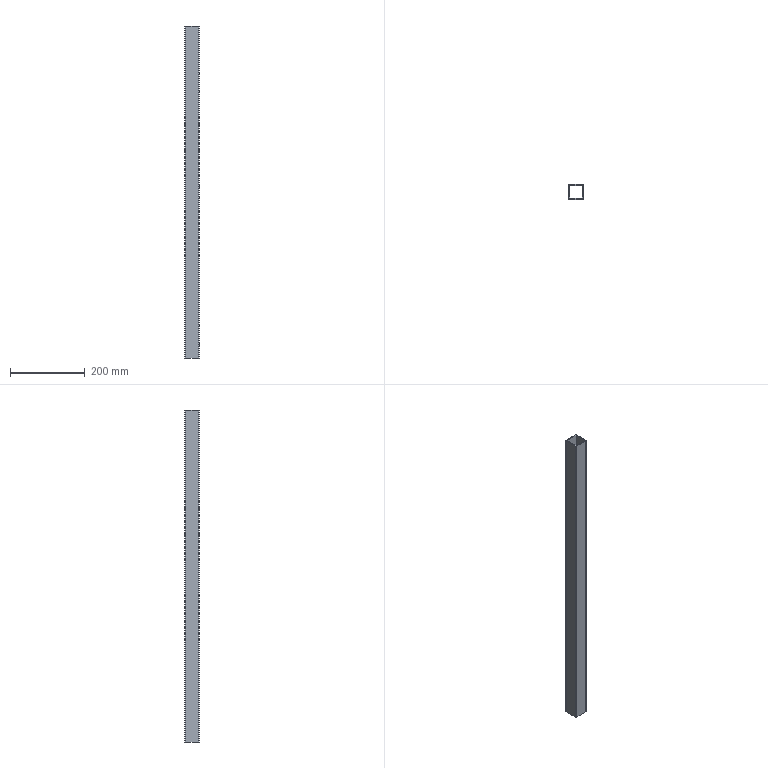Part | STEP file | X77-04201 | 1 solid | 26 faces | box 40 x 40 x 890 mm | volume 388035 mm3 | cylinder 16 | plane 10 | commonest cylinder face diameters 4.2 x12 6 x4
STEP:
#1=CARTESIAN_POINT('',(17.,12.,83.8));
#2=VERTEX_POINT('',#1);
#3=CARTESIAN_POINT('',(17.,12.,88.));
#4=VERTEX_POINT('',#3);
#5=CARTESIAN_POINT('',(17.,12.,85.9));
#6=DIRECTION('',(-1.,0.,0.));
#7=DIRECTION('',(0.,0.,1.));
#8=AXIS2_PLACEMENT_3D('',#5,#6,#7);
#9=CIRCLE('',#8,2.1);
#10=EDGE_CURVE('',#2,#4,#9,.T.);
#11=ORIENTED_EDGE('',*,*,#10,.T.);
#12=CARTESIAN_POINT('',(20.,12.,88.));
#13=VERTEX_POINT('',#12);
#14=CARTESIAN_POINT('',(20.,12.,88.));
#15=DIRECTION('',(1.,0.,0.));
#16=VECTOR('',#15,1000.);
#17=LINE('',#14,#16);
#18=EDGE_CURVE('',#4,#13,#17,.T.);
#19=ORIENTED_EDGE('',*,*,#18,.T.);
#20=CARTESIAN_POINT('',(20.,12.,83.8));
#21=VERTEX_POINT('',#20);
#22=CARTESIAN_POINT('',(20.,12.,85.9));
#23=DIRECTION('',(1.,0.,0.));
#24=DIRECTION('',(0.,0.,-1.));
#25=AXIS2_PLACEMENT_3D('',#22,#23,#24);
#26=CIRCLE('',#25,2.1);
#27=EDGE_CURVE('',#13,#21,#26,.T.);
#28=ORIENTED_EDGE('',*,*,#27,.T.);
#29=CARTESIAN_POINT('',(20.,12.,83.8));
#30=DIRECTION('',(1.,0.,0.));
#31=VECTOR('',#30,1000.);
#32=LINE('',#29,#31);
#33=EDGE_CURVE('',#2,#21,#32,.T.);
#34=ORIENTED_EDGE('',*,*,#33,.F.);
#35=EDGE_LOOP('',(#11,#19,#28,#34));
#36=FACE_OUTER_BOUND('',#35,.T.);
#37=CARTESIAN_POINT('',(20.,12.,85.9));
#38=DIRECTION('',(1.,0.,0.));
#39=DIRECTION('',(0.,0.,-1.));
#40=AXIS2_PLACEMENT_3D('',#37,#38,#39);
#41=CYLINDRICAL_SURFACE('',#40,2.1);
#42=ADVANCED_FACE('',(#36),#41,.F.);
#43=CARTESIAN_POINT('',(17.,-12.,33.8));
#44=VERTEX_POINT('',#43);
#45=CARTESIAN_POINT('',(17.,-12.,38.));
#46=VERTEX_POINT('',#45);
#47=CARTESIAN_POINT('',(17.,-12.,35.9));
#48=DIRECTION('',(-1.,0.,0.));
#49=DIRECTION('',(0.,0.,1.));
#50=AXIS2_PLACEMENT_3D('',#47,#48,#49);
#51=CIRCLE('',#50,2.1);
#52=EDGE_CURVE('',#44,#46,#51,.T.);
#53=ORIENTED_EDGE('',*,*,#52,.T.);
#54=CARTESIAN_POINT('',(20.,-12.,38.));
#55=VERTEX_POINT('',#54);
#56=CARTESIAN_POINT('',(20.,-12.,38.));
#57=DIRECTION('',(1.,0.,0.));
#58=VECTOR('',#57,1000.);
#59=LINE('',#56,#58);
#60=EDGE_CURVE('',#46,#55,#59,.T.);
#61=ORIENTED_EDGE('',*,*,#60,.T.);
#62=CARTESIAN_POINT('',(20.,-12.,33.8));
#63=VERTEX_POINT('',#62);
#64=CARTESIAN_POINT('',(20.,-12.,35.9));
#65=DIRECTION('',(1.,0.,0.));
#66=DIRECTION('',(0.,0.,-1.));
#67=AXIS2_PLACEMENT_3D('',#64,#65,#66);
#68=CIRCLE('',#67,2.1);
#69=EDGE_CURVE('',#55,#63,#68,.T.);
#70=ORIENTED_EDGE('',*,*,#69,.T.);
#71=CARTESIAN_POINT('',(20.,-12.,33.8));
#72=DIRECTION('',(1.,0.,0.));
#73=VECTOR('',#72,1000.);
#74=LINE('',#71,#73);
#75=EDGE_CURVE('',#44,#63,#74,.T.);
#76=ORIENTED_EDGE('',*,*,#75,.F.);
#77=EDGE_LOOP('',(#53,#61,#70,#76));
#78=FACE_OUTER_BOUND('',#77,.T.);
#79=CARTESIAN_POINT('',(20.,-12.,35.9));
#80=DIRECTION('',(1.,0.,0.));
#81=DIRECTION('',(0.,0.,-1.));
#82=AXIS2_PLACEMENT_3D('',#79,#80,#81);
#83=CYLINDRICAL_SURFACE('',#82,2.1);
#84=ADVANCED_FACE('',(#78),#83,.F.);
#85=CARTESIAN_POINT('',(17.,12.,762.));
#86=VERTEX_POINT('',#85);
#87=CARTESIAN_POINT('',(17.,12.,766.2));
#88=VERTEX_POINT('',#87);
#89=CARTESIAN_POINT('',(17.,12.,764.1));
#90=DIRECTION('',(-1.,0.,0.));
#91=DIRECTION('',(0.,0.,1.));
#92=AXIS2_PLACEMENT_3D('',#89,#90,#91);
#93=CIRCLE('',#92,2.1);
#94=EDGE_CURVE('',#86,#88,#93,.T.);
#95=ORIENTED_EDGE('',*,*,#94,.T.);
#96=CARTESIAN_POINT('',(20.,12.,766.2));
#97=VERTEX_POINT('',#96);
#98=CARTESIAN_POINT('',(20.,12.,766.2));
#99=DIRECTION('',(1.,0.,0.));
#100=VECTOR('',#99,1000.);
#101=LINE('',#98,#100);
#102=EDGE_CURVE('',#88,#97,#101,.T.);
#103=ORIENTED_EDGE('',*,*,#102,.T.);
#104=CARTESIAN_POINT('',(20.,12.,762.));
#105=VERTEX_POINT('',#104);
#106=CARTESIAN_POINT('',(20.,12.,764.1));
#107=DIRECTION('',(1.,0.,0.));
#108=DIRECTION('',(0.,0.,-1.));
#109=AXIS2_PLACEMENT_3D('',#106,#107,#108);
#110=CIRCLE('',#109,2.1);
#111=EDGE_CURVE('',#97,#105,#110,.T.);
#112=ORIENTED_EDGE('',*,*,#111,.T.);
#113=CARTESIAN_POINT('',(20.,12.,762.));
#114=DIRECTION('',(1.,0.,0.));
#115=VECTOR('',#114,1000.);
#116=LINE('',#113,#115);
#117=EDGE_CURVE('',#86,#105,#116,.T.);
#118=ORIENTED_EDGE('',*,*,#117,.F.);
#119=EDGE_LOOP('',(#95,#103,#112,#118));
#120=FACE_OUTER_BOUND('',#119,.T.);
#121=CARTESIAN_POINT('',(20.,12.,764.1));
#122=DIRECTION('',(1.,0.,0.));
#123=DIRECTION('',(0.,0.,-1.));
#124=AXIS2_PLACEMENT_3D('',#121,#122,#123);
#125=CYLINDRICAL_SURFACE('',#124,2.1);
#126=ADVANCED_FACE('',(#120),#125,.F.);
#127=CARTESIAN_POINT('',(17.,-12.,712.));
#128=VERTEX_POINT('',#127);
#129=CARTESIAN_POINT('',(17.,-12.,716.2));
#130=VERTEX_POINT('',#129);
#131=CARTESIAN_POINT('',(17.,-12.,714.1));
#132=DIRECTION('',(-1.,0.,0.));
#133=DIRECTION('',(0.,0.,1.));
#134=AXIS2_PLACEMENT_3D('',#131,#132,#133);
#135=CIRCLE('',#134,2.1);
#136=EDGE_CURVE('',#128,#130,#135,.T.);
#137=ORIENTED_EDGE('',*,*,#136,.T.);
#138=CARTESIAN_POINT('',(20.,-12.,716.2));
#139=VERTEX_POINT('',#138);
#140=CARTESIAN_POINT('',(20.,-12.,716.2));
#141=DIRECTION('',(1.,0.,0.));
#142=VECTOR('',#141,1000.);
#143=LINE('',#140,#142);
#144=EDGE_CURVE('',#130,#139,#143,.T.);
#145=ORIENTED_EDGE('',*,*,#144,.T.);
#146=CARTESIAN_POINT('',(20.,-12.,712.));
#147=VERTEX_POINT('',#146);
#148=CARTESIAN_POINT('',(20.,-12.,714.1));
#149=DIRECTION('',(1.,0.,0.));
#150=DIRECTION('',(0.,0.,-1.));
#151=AXIS2_PLACEMENT_3D('',#148,#149,#150);
#152=CIRCLE('',#151,2.1);
#153=EDGE_CURVE('',#139,#147,#152,.T.);
#154=ORIENTED_EDGE('',*,*,#153,.T.);
#155=CARTESIAN_POINT('',(20.,-12.,712.));
#156=DIRECTION('',(1.,0.,0.));
#157=VECTOR('',#156,1000.);
#158=LINE('',#155,#157);
#159=EDGE_CURVE('',#128,#147,#158,.T.);
#160=ORIENTED_EDGE('',*,*,#159,.F.);
#161=EDGE_LOOP('',(#137,#145,#154,#160));
#162=FACE_OUTER_BOUND('',#161,.T.);
#163=CARTESIAN_POINT('',(20.,-12.,714.1));
#164=DIRECTION('',(1.,0.,0.));
#165=DIRECTION('',(0.,0.,-1.));
#166=AXIS2_PLACEMENT_3D('',#163,#164,#165);
#167=CYLINDRICAL_SURFACE('',#166,2.1);
#168=ADVANCED_FACE('',(#162),#167,.F.);
#169=CARTESIAN_POINT('',(17.,0.,457.9));
#170=VERTEX_POINT('',#169);
#171=CARTESIAN_POINT('',(17.,0.,462.1));
#172=VERTEX_POINT('',#171);
#173=CARTESIAN_POINT('',(17.,0.,460.));
#174=DIRECTION('',(-1.,0.,0.));
#175=DIRECTION('',(0.,0.,1.));
#176=AXIS2_PLACEMENT_3D('',#173,#174,#175);
#177=CIRCLE('',#176,2.1);
#178=EDGE_CURVE('',#170,#172,#177,.T.);
#179=ORIENTED_EDGE('',*,*,#178,.T.);
#180=CARTESIAN_POINT('',(20.,0.,462.1));
#181=VERTEX_POINT('',#180);
#182=CARTESIAN_POINT('',(20.,0.,462.1));
#183=DIRECTION('',(1.,0.,0.));
#184=VECTOR('',#183,1000.);
#185=LINE('',#182,#184);
#186=EDGE_CURVE('',#172,#181,#185,.T.);
#187=ORIENTED_EDGE('',*,*,#186,.T.);
#188=CARTESIAN_POINT('',(20.,0.,457.9));
#189=VERTEX_POINT('',#188);
#190=CARTESIAN_POINT('',(20.,0.,460.));
#191=DIRECTION('',(1.,0.,0.));
#192=DIRECTION('',(0.,0.,-1.));
#193=AXIS2_PLACEMENT_3D('',#190,#191,#192);
#194=CIRCLE('',#193,2.1);
#195=EDGE_CURVE('',#181,#189,#194,.T.);
#196=ORIENTED_EDGE('',*,*,#195,.T.);
#197=CARTESIAN_POINT('',(20.,0.,457.9));
#198=DIRECTION('',(1.,0.,0.));
#199=VECTOR('',#198,1000.);
#200=LINE('',#197,#199);
#201=EDGE_CURVE('',#170,#189,#200,.T.);
#202=ORIENTED_EDGE('',*,*,#201,.F.);
#203=EDGE_LOOP('',(#179,#187,#196,#202));
#204=FACE_OUTER_BOUND('',#203,.T.);
#205=CARTESIAN_POINT('',(20.,0.,460.));
#206=DIRECTION('',(1.,0.,0.));
#207=DIRECTION('',(0.,0.,-1.));
#208=AXIS2_PLACEMENT_3D('',#205,#206,#207);
#209=CYLINDRICAL_SURFACE('',#208,2.1);
#210=ADVANCED_FACE('',(#204),#209,.F.);
#211=CARTESIAN_POINT('',(17.,0.,427.9));
#212=VERTEX_POINT('',#211);
#213=CARTESIAN_POINT('',(17.,0.,432.1));
#214=VERTEX_POINT('',#213);
#215=CARTESIAN_POINT('',(17.,0.,430.));
#216=DIRECTION('',(-1.,0.,0.));
#217=DIRECTION('',(0.,0.,1.));
#218=AXIS2_PLACEMENT_3D('',#215,#216,#217);
#219=CIRCLE('',#218,2.1);
#220=EDGE_CURVE('',#212,#214,#219,.T.);
#221=ORIENTED_EDGE('',*,*,#220,.T.);
#222=CARTESIAN_POINT('',(20.,0.,432.1));
#223=VERTEX_POINT('',#222);
#224=CARTESIAN_POINT('',(20.,0.,432.1));
#225=DIRECTION('',(1.,0.,0.));
#226=VECTOR('',#225,1000.);
#227=LINE('',#224,#226);
#228=EDGE_CURVE('',#214,#223,#227,.T.);
#229=ORIENTED_EDGE('',*,*,#228,.T.);
#230=CARTESIAN_POINT('',(20.,0.,427.9));
#231=VERTEX_POINT('',#230);
#232=CARTESIAN_POINT('',(20.,0.,430.));
#233=DIRECTION('',(1.,0.,0.));
#234=DIRECTION('',(0.,0.,-1.));
#235=AXIS2_PLACEMENT_3D('',#232,#233,#234);
#236=CIRCLE('',#235,2.1);
#237=EDGE_CURVE('',#223,#231,#236,.T.);
#238=ORIENTED_EDGE('',*,*,#237,.T.);
#239=CARTESIAN_POINT('',(20.,0.,427.9));
#240=DIRECTION('',(1.,0.,0.));
#241=VECTOR('',#240,1000.);
#242=LINE('',#239,#241);
#243=EDGE_CURVE('',#212,#231,#242,.T.);
#244=ORIENTED_EDGE('',*,*,#243,.F.);
#245=EDGE_LOOP('',(#221,#229,#238,#244));
#246=FACE_OUTER_BOUND('',#245,.T.);
#247=CARTESIAN_POINT('',(20.,0.,430.));
#248=DIRECTION('',(1.,0.,0.));
#249=DIRECTION('',(0.,0.,-1.));
#250=AXIS2_PLACEMENT_3D('',#247,#248,#249);
#251=CYLINDRICAL_SURFACE('',#250,2.1);
#252=ADVANCED_FACE('',(#246),#251,.F.);
#253=CARTESIAN_POINT('',(-20.,-17.,890.));
#254=VERTEX_POINT('',#253);
#255=CARTESIAN_POINT('',(-17.,-20.,890.));
#256=VERTEX_POINT('',#255);
#257=CARTESIAN_POINT('',(-17.,-17.,890.));
#258=DIRECTION('',(0.,0.,1.));
#259=DIRECTION('',(-1.,0.,0.));
#260=AXIS2_PLACEMENT_3D('',#257,#258,#259);
#261=CIRCLE('',#260,3.);
#262=EDGE_CURVE('',#254,#256,#261,.T.);
#263=ORIENTED_EDGE('',*,*,#262,.T.);
#264=CARTESIAN_POINT('',(17.,-20.,890.));
#265=VERTEX_POINT('',#264);
#266=CARTESIAN_POINT('',(-17.,-20.,890.));
#267=DIRECTION('',(1.,0.,0.));
#268=VECTOR('',#267,1000.);
#269=LINE('',#266,#268);
#270=EDGE_CURVE('',#256,#265,#269,.T.);
#271=ORIENTED_EDGE('',*,*,#270,.T.);
#272=CARTESIAN_POINT('',(20.,-17.,890.));
#273=VERTEX_POINT('',#272);
#274=CARTESIAN_POINT('',(17.,-17.,890.));
#275=DIRECTION('',(0.,0.,1.));
#276=DIRECTION('',(-1.,0.,0.));
#277=AXIS2_PLACEMENT_3D('',#274,#275,#276);
#278=CIRCLE('',#277,3.);
#279=EDGE_CURVE('',#265,#273,#278,.T.);
#280=ORIENTED_EDGE('',*,*,#279,.T.);
#281=CARTESIAN_POINT('',(20.,17.,890.));
#282=VERTEX_POINT('',#281);
#283=CARTESIAN_POINT('',(20.,-17.,890.));
#284=DIRECTION('',(0.,1.,0.));
#285=VECTOR('',#284,1000.);
#286=LINE('',#283,#285);
#287=EDGE_CURVE('',#273,#282,#286,.T.);
#288=ORIENTED_EDGE('',*,*,#287,.T.);
#289=CARTESIAN_POINT('',(17.,20.,890.));
#290=VERTEX_POINT('',#289);
#291=CARTESIAN_POINT('',(17.,17.,890.));
#292=DIRECTION('',(0.,0.,1.));
#293=DIRECTION('',(1.,0.,0.));
#294=AXIS2_PLACEMENT_3D('',#291,#292,#293);
#295=CIRCLE('',#294,3.);
#296=EDGE_CURVE('',#282,#290,#295,.T.);
#297=ORIENTED_EDGE('',*,*,#296,.T.);
#298=CARTESIAN_POINT('',(-17.,20.,890.));
#299=VERTEX_POINT('',#298);
#300=CARTESIAN_POINT('',(-17.,20.,890.));
#301=DIRECTION('',(-1.,0.,0.));
#302=VECTOR('',#301,1000.);
#303=LINE('',#300,#302);
#304=EDGE_CURVE('',#290,#299,#303,.T.);
#305=ORIENTED_EDGE('',*,*,#304,.T.);
#306=CARTESIAN_POINT('',(-20.,17.,890.));
#307=VERTEX_POINT('',#306);
#308=CARTESIAN_POINT('',(-17.,17.,890.));
#309=DIRECTION('',(0.,0.,1.));
#310=DIRECTION('',(1.,0.,0.));
#311=AXIS2_PLACEMENT_3D('',#308,#309,#310);
#312=CIRCLE('',#311,3.);
#313=EDGE_CURVE('',#299,#307,#312,.T.);
#314=ORIENTED_EDGE('',*,*,#313,.T.);
#315=CARTESIAN_POINT('',(-20.,-17.,890.));
#316=DIRECTION('',(0.,-1.,0.));
#317=VECTOR('',#316,1000.);
#318=LINE('',#315,#317);
#319=EDGE_CURVE('',#307,#254,#318,.T.);
#320=ORIENTED_EDGE('',*,*,#319,.T.);
#321=EDGE_LOOP('',(#263,#271,#280,#288,#297,#305,#314,#320));
#322=FACE_OUTER_BOUND('',#321,.T.);
#323=CARTESIAN_POINT('',(17.,-17.,890.));
#324=VERTEX_POINT('',#323);
#325=CARTESIAN_POINT('',(17.,17.,890.));
#326=VERTEX_POINT('',#325);
#327=CARTESIAN_POINT('',(17.,-17.,890.));
#328=DIRECTION('',(0.,1.,0.));
#329=VECTOR('',#328,1000.);
#330=LINE('',#327,#329);
#331=EDGE_CURVE('',#324,#326,#330,.T.);
#332=ORIENTED_EDGE('',*,*,#331,.F.);
#333=CARTESIAN_POINT('',(-17.,-17.,890.));
#334=VERTEX_POINT('',#333);
#335=CARTESIAN_POINT('',(-17.,-17.,890.));
#336=DIRECTION('',(1.,0.,0.));
#337=VECTOR('',#336,1000.);
#338=LINE('',#335,#337);
#339=EDGE_CURVE('',#334,#324,#338,.T.);
#340=ORIENTED_EDGE('',*,*,#339,.F.);
#341=CARTESIAN_POINT('',(-17.,17.,890.));
#342=VERTEX_POINT('',#341);
#343=CARTESIAN_POINT('',(-17.,-17.,890.));
#344=DIRECTION('',(0.,-1.,0.));
#345=VECTOR('',#344,1000.);
#346=LINE('',#343,#345);
#347=EDGE_CURVE('',#342,#334,#346,.T.);
#348=ORIENTED_EDGE('',*,*,#347,.F.);
#349=CARTESIAN_POINT('',(-17.,17.,890.));
#350=DIRECTION('',(-1.,0.,0.));
#351=VECTOR('',#350,1000.);
#352=LINE('',#349,#351);
#353=EDGE_CURVE('',#326,#342,#352,.T.);
#354=ORIENTED_EDGE('',*,*,#353,.F.);
#355=EDGE_LOOP('',(#332,#340,#348,#354));
#356=FACE_BOUND('',#355,.T.);
#357=CARTESIAN_POINT('',(-17.,-17.,890.));
#358=DIRECTION('',(0.,0.,-1.));
#359=DIRECTION('',(-1.,0.,0.));
#360=AXIS2_PLACEMENT_3D('',#357,#358,#359);
#361=PLANE('',#360);
#362=ADVANCED_FACE('',(#322,#356),#361,.F.);
#363=CARTESIAN_POINT('',(-20.,-17.,0.));
#364=VERTEX_POINT('',#363);
#365=CARTESIAN_POINT('',(-17.,-20.,0.));
#366=VERTEX_POINT('',#365);
#367=CARTESIAN_POINT('',(-17.,-17.,0.));
#368=DIRECTION('',(0.,0.,1.));
#369=DIRECTION('',(-1.,0.,0.));
#370=AXIS2_PLACEMENT_3D('',#367,#368,#369);
#371=CIRCLE('',#370,3.);
#372=EDGE_CURVE('',#364,#366,#371,.T.);
#373=ORIENTED_EDGE('',*,*,#372,.F.);
#374=CARTESIAN_POINT('',(-20.,17.,0.));
#375=VERTEX_POINT('',#374);
#376=CARTESIAN_POINT('',(-20.,-17.,0.));
#377=DIRECTION('',(0.,-1.,0.));
#378=VECTOR('',#377,1000.);
#379=LINE('',#376,#378);
#380=EDGE_CURVE('',#375,#364,#379,.T.);
#381=ORIENTED_EDGE('',*,*,#380,.F.);
#382=CARTESIAN_POINT('',(-17.,20.,0.));
#383=VERTEX_POINT('',#382);
#384=CARTESIAN_POINT('',(-17.,17.,0.));
#385=DIRECTION('',(0.,0.,1.));
#386=DIRECTION('',(1.,0.,0.));
#387=AXIS2_PLACEMENT_3D('',#384,#385,#386);
#388=CIRCLE('',#387,3.);
#389=EDGE_CURVE('',#383,#375,#388,.T.);
#390=ORIENTED_EDGE('',*,*,#389,.F.);
#391=CARTESIAN_POINT('',(17.,20.,0.));
#392=VERTEX_POINT('',#391);
#393=CARTESIAN_POINT('',(-17.,20.,0.));
#394=DIRECTION('',(-1.,0.,0.));
#395=VECTOR('',#394,1000.);
#396=LINE('',#393,#395);
#397=EDGE_CURVE('',#392,#383,#396,.T.);
#398=ORIENTED_EDGE('',*,*,#397,.F.);
#399=CARTESIAN_POINT('',(20.,17.,0.));
#400=VERTEX_POINT('',#399);
#401=CARTESIAN_POINT('',(17.,17.,0.));
#402=DIRECTION('',(0.,0.,1.));
#403=DIRECTION('',(1.,0.,0.));
#404=AXIS2_PLACEMENT_3D('',#401,#402,#403);
#405=CIRCLE('',#404,3.);
#406=EDGE_CURVE('',#400,#392,#405,.T.);
#407=ORIENTED_EDGE('',*,*,#406,.F.);
#408=CARTESIAN_POINT('',(20.,-17.,0.));
#409=VERTEX_POINT('',#408);
#410=CARTESIAN_POINT('',(20.,-17.,0.));
#411=DIRECTION('',(0.,1.,0.));
#412=VECTOR('',#411,1000.);
#413=LINE('',#410,#412);
#414=EDGE_CURVE('',#409,#400,#413,.T.);
#415=ORIENTED_EDGE('',*,*,#414,.F.);
#416=CARTESIAN_POINT('',(17.,-20.,0.));
#417=VERTEX_POINT('',#416);
#418=CARTESIAN_POINT('',(17.,-17.,0.));
#419=DIRECTION('',(0.,0.,1.));
#420=DIRECTION('',(-1.,0.,0.));
#421=AXIS2_PLACEMENT_3D('',#418,#419,#420);
#422=CIRCLE('',#421,3.);
#423=EDGE_CURVE('',#417,#409,#422,.T.);
#424=ORIENTED_EDGE('',*,*,#423,.F.);
#425=CARTESIAN_POINT('',(-17.,-20.,0.));
#426=DIRECTION('',(1.,0.,0.));
#427=VECTOR('',#426,1000.);
#428=LINE('',#425,#427);
#429=EDGE_CURVE('',#366,#417,#428,.T.);
#430=ORIENTED_EDGE('',*,*,#429,.F.);
#431=EDGE_LOOP('',(#373,#381,#390,#398,#407,#415,#424,#430));
#432=FACE_OUTER_BOUND('',#431,.T.);
#433=CARTESIAN_POINT('',(-17.,-17.,0.));
#434=VERTEX_POINT('',#433);
#435=CARTESIAN_POINT('',(17.,-17.,0.));
#436=VERTEX_POINT('',#435);
#437=CARTESIAN_POINT('',(-17.,-17.,0.));
#438=DIRECTION('',(1.,0.,0.));
#439=VECTOR('',#438,1000.);
#440=LINE('',#437,#439);
#441=EDGE_CURVE('',#434,#436,#440,.T.);
#442=ORIENTED_EDGE('',*,*,#441,.T.);
#443=CARTESIAN_POINT('',(17.,17.,0.));
#444=VERTEX_POINT('',#443);
#445=CARTESIAN_POINT('',(17.,-17.,0.));
#446=DIRECTION('',(0.,1.,0.));
#447=VECTOR('',#446,1000.);
#448=LINE('',#445,#447);
#449=EDGE_CURVE('',#436,#444,#448,.T.);
#450=ORIENTED_EDGE('',*,*,#449,.T.);
#451=CARTESIAN_POINT('',(-17.,17.,0.));
#452=VERTEX_POINT('',#451);
#453=CARTESIAN_POINT('',(-17.,17.,0.));
#454=DIRECTION('',(-1.,0.,0.));
#455=VECTOR('',#454,1000.);
#456=LINE('',#453,#455);
#457=EDGE_CURVE('',#444,#452,#456,.T.);
#458=ORIENTED_EDGE('',*,*,#457,.T.);
#459=CARTESIAN_POINT('',(-17.,-17.,0.));
#460=DIRECTION('',(0.,-1.,0.));
#461=VECTOR('',#460,1000.);
#462=LINE('',#459,#461);
#463=EDGE_CURVE('',#452,#434,#462,.T.);
#464=ORIENTED_EDGE('',*,*,#463,.T.);
#465=EDGE_LOOP('',(#442,#450,#458,#464));
#466=FACE_BOUND('',#465,.T.);
#467=CARTESIAN_POINT('',(-17.,-17.,0.));
#468=DIRECTION('',(0.,0.,-1.));
#469=DIRECTION('',(-1.,0.,0.));
#470=AXIS2_PLACEMENT_3D('',#467,#468,#469);
#471=PLANE('',#470);
#472=ADVANCED_FACE('',(#432,#466),#471,.T.);
#473=ORIENTED_EDGE('',*,*,#372,.T.);
#474=CARTESIAN_POINT('',(-17.,-20.,890.));
#475=DIRECTION('',(0.,0.,-1.));
#476=VECTOR('',#475,1000.);
#477=LINE('',#474,#476);
#478=EDGE_CURVE('',#256,#366,#477,.T.);
#479=ORIENTED_EDGE('',*,*,#478,.F.);
#480=ORIENTED_EDGE('',*,*,#262,.F.);
#481=CARTESIAN_POINT('',(-20.,-17.,890.));
#482=DIRECTION('',(0.,0.,-1.));
#483=VECTOR('',#482,1000.);
#484=LINE('',#481,#483);
#485=EDGE_CURVE('',#254,#364,#484,.T.);
#486=ORIENTED_EDGE('',*,*,#485,.T.);
#487=EDGE_LOOP('',(#473,#479,#480,#486));
#488=FACE_OUTER_BOUND('',#487,.T.);
#489=CARTESIAN_POINT('',(-17.,-17.,890.));
#490=DIRECTION('',(0.,0.,-1.));
#491=DIRECTION('',(-1.,0.,0.));
#492=AXIS2_PLACEMENT_3D('',#489,#490,#491);
#493=CYLINDRICAL_SURFACE('',#492,3.);
#494=ADVANCED_FACE('',(#488),#493,.T.);
#495=ORIENTED_EDGE('',*,*,#429,.T.);
#496=CARTESIAN_POINT('',(17.,-20.,890.));
#497=DIRECTION('',(0.,0.,-1.));
#498=VECTOR('',#497,1000.);
#499=LINE('',#496,#498);
#500=EDGE_CURVE('',#265,#417,#499,.T.);
#501=ORIENTED_EDGE('',*,*,#500,.F.);
#502=ORIENTED_EDGE('',*,*,#270,.F.);
#503=ORIENTED_EDGE('',*,*,#478,.T.);
#504=EDGE_LOOP('',(#495,#501,#502,#503));
#505=FACE_OUTER_BOUND('',#504,.T.);
#506=CARTESIAN_POINT('',(-17.,-20.,890.));
#507=DIRECTION('',(0.,1.,0.));
#508=DIRECTION('',(0.,0.,1.));
#509=AXIS2_PLACEMENT_3D('',#506,#507,#508);
#510=PLANE('',#509);
#511=ADVANCED_FACE('',(#505),#510,.F.);
#512=ORIENTED_EDGE('',*,*,#423,.T.);
#513=CARTESIAN_POINT('',(20.,-17.,890.));
#514=DIRECTION('',(0.,0.,-1.));
#515=VECTOR('',#514,1000.);
#516=LINE('',#513,#515);
#517=EDGE_CURVE('',#273,#409,#516,.T.);
#518=ORIENTED_EDGE('',*,*,#517,.F.);
#519=ORIENTED_EDGE('',*,*,#279,.F.);
#520=ORIENTED_EDGE('',*,*,#500,.T.);
#521=EDGE_LOOP('',(#512,#518,#519,#520));
#522=FACE_OUTER_BOUND('',#521,.T.);
#523=CARTESIAN_POINT('',(17.,-17.,890.));
#524=DIRECTION('',(0.,0.,-1.));
#525=DIRECTION('',(-1.,0.,0.));
#526=AXIS2_PLACEMENT_3D('',#523,#524,#525);
#527=CYLINDRICAL_SURFACE('',#526,3.);
#528=ADVANCED_FACE('',(#522),#527,.T.);
#529=CARTESIAN_POINT('',(20.,12.,85.9));
#530=DIRECTION('',(1.,0.,0.));
#531=DIRECTION('',(0.,0.,-1.));
#532=AXIS2_PLACEMENT_3D('',#529,#530,#531);
#533=CIRCLE('',#532,2.1);
#534=EDGE_CURVE('',#21,#13,#533,.T.);
#535=ORIENTED_EDGE('',*,*,#534,.F.);
#536=ORIENTED_EDGE('',*,*,#27,.F.);
#537=EDGE_LOOP('',(#535,#536));
#538=FACE_BOUND('',#537,.T.);
#539=CARTESIAN_POINT('',(20.,-12.,35.9));
#540=DIRECTION('',(1.,0.,0.));
#541=DIRECTION('',(0.,0.,-1.));
#542=AXIS2_PLACEMENT_3D('',#539,#540,#541);
#543=CIRCLE('',#542,2.1);
#544=EDGE_CURVE('',#63,#55,#543,.T.);
#545=ORIENTED_EDGE('',*,*,#544,.F.);
#546=ORIENTED_EDGE('',*,*,#69,.F.);
#547=EDGE_LOOP('',(#545,#546));
#548=FACE_BOUND('',#547,.T.);
#549=CARTESIAN_POINT('',(20.,12.,764.1));
#550=DIRECTION('',(1.,0.,0.));
#551=DIRECTION('',(0.,0.,-1.));
#552=AXIS2_PLACEMENT_3D('',#549,#550,#551);
#553=CIRCLE('',#552,2.1);
#554=EDGE_CURVE('',#105,#97,#553,.T.);
#555=ORIENTED_EDGE('',*,*,#554,.F.);
#556=ORIENTED_EDGE('',*,*,#111,.F.);
#557=EDGE_LOOP('',(#555,#556));
#558=FACE_BOUND('',#557,.T.);
#559=CARTESIAN_POINT('',(20.,-12.,714.1));
#560=DIRECTION('',(1.,0.,0.));
#561=DIRECTION('',(0.,0.,-1.));
#562=AXIS2_PLACEMENT_3D('',#559,#560,#561);
#563=CIRCLE('',#562,2.1);
#564=EDGE_CURVE('',#147,#139,#563,.T.);
#565=ORIENTED_EDGE('',*,*,#564,.F.);
#566=ORIENTED_EDGE('',*,*,#153,.F.);
#567=EDGE_LOOP('',(#565,#566));
#568=FACE_BOUND('',#567,.T.);
#569=CARTESIAN_POINT('',(20.,0.,460.));
#570=DIRECTION('',(1.,0.,0.));
#571=DIRECTION('',(0.,0.,-1.));
#572=AXIS2_PLACEMENT_3D('',#569,#570,#571);
#573=CIRCLE('',#572,2.1);
#574=EDGE_CURVE('',#189,#181,#573,.T.);
#575=ORIENTED_EDGE('',*,*,#574,.F.);
#576=ORIENTED_EDGE('',*,*,#195,.F.);
#577=EDGE_LOOP('',(#575,#576));
#578=FACE_BOUND('',#577,.T.);
#579=CARTESIAN_POINT('',(20.,0.,430.));
#580=DIRECTION('',(1.,0.,0.));
#581=DIRECTION('',(0.,0.,-1.));
#582=AXIS2_PLACEMENT_3D('',#579,#580,#581);
#583=CIRCLE('',#582,2.1);
#584=EDGE_CURVE('',#231,#223,#583,.T.);
#585=ORIENTED_EDGE('',*,*,#584,.F.);
#586=ORIENTED_EDGE('',*,*,#237,.F.);
#587=EDGE_LOOP('',(#585,#586));
#588=FACE_BOUND('',#587,.T.);
#589=ORIENTED_EDGE('',*,*,#414,.T.);
#590=CARTESIAN_POINT('',(20.,17.,890.));
#591=DIRECTION('',(0.,0.,-1.));
#592=VECTOR('',#591,1000.);
#593=LINE('',#590,#592);
#594=EDGE_CURVE('',#282,#400,#593,.T.);
#595=ORIENTED_EDGE('',*,*,#594,.F.);
#596=ORIENTED_EDGE('',*,*,#287,.F.);
#597=ORIENTED_EDGE('',*,*,#517,.T.);
#598=EDGE_LOOP('',(#589,#595,#596,#597));
#599=FACE_OUTER_BOUND('',#598,.T.);
#600=CARTESIAN_POINT('',(20.,-17.,890.));
#601=DIRECTION('',(-1.,0.,0.));
#602=DIRECTION('',(0.,0.,1.));
#603=AXIS2_PLACEMENT_3D('',#600,#601,#602);
#604=PLANE('',#603);
#605=ADVANCED_FACE('',(#538,#548,#558,#568,#578,#588,#599),#604,.F.);
#606=ORIENTED_EDGE('',*,*,#406,.T.);
#607=CARTESIAN_POINT('',(17.,20.,890.));
#608=DIRECTION('',(0.,0.,-1.));
#609=VECTOR('',#608,1000.);
#610=LINE('',#607,#609);
#611=EDGE_CURVE('',#290,#392,#610,.T.);
#612=ORIENTED_EDGE('',*,*,#611,.F.);
#613=ORIENTED_EDGE('',*,*,#296,.F.);
#614=ORIENTED_EDGE('',*,*,#594,.T.);
#615=EDGE_LOOP('',(#606,#612,#613,#614));
#616=FACE_OUTER_BOUND('',#615,.T.);
#617=CARTESIAN_POINT('',(17.,17.,890.));
#618=DIRECTION('',(0.,0.,-1.));
#619=DIRECTION('',(-1.,0.,0.));
#620=AXIS2_PLACEMENT_3D('',#617,#618,#619);
#621=CYLINDRICAL_SURFACE('',#620,3.);
#622=ADVANCED_FACE('',(#616),#621,.T.);
#623=ORIENTED_EDGE('',*,*,#397,.T.);
#624=CARTESIAN_POINT('',(-17.,20.,890.));
#625=DIRECTION('',(0.,0.,-1.));
#626=VECTOR('',#625,1000.);
#627=LINE('',#624,#626);
#628=EDGE_CURVE('',#299,#383,#627,.T.);
#629=ORIENTED_EDGE('',*,*,#628,.F.);
#630=ORIENTED_EDGE('',*,*,#304,.F.);
#631=ORIENTED_EDGE('',*,*,#611,.T.);
#632=EDGE_LOOP('',(#623,#629,#630,#631));
#633=FACE_OUTER_BOUND('',#632,.T.);
#634=CARTESIAN_POINT('',(-17.,20.,890.));
#635=DIRECTION('',(0.,-1.,0.));
#636=DIRECTION('',(0.,0.,-1.));
#637=AXIS2_PLACEMENT_3D('',#634,#635,#636);
#638=PLANE('',#637);
#639=ADVANCED_FACE('',(#633),#638,.F.);
#640=ORIENTED_EDGE('',*,*,#389,.T.);
#641=CARTESIAN_POINT('',(-20.,17.,890.));
#642=DIRECTION('',(0.,0.,-1.));
#643=VECTOR('',#642,1000.);
#644=LINE('',#641,#643);
#645=EDGE_CURVE('',#307,#375,#644,.T.);
#646=ORIENTED_EDGE('',*,*,#645,.F.);
#647=ORIENTED_EDGE('',*,*,#313,.F.);
#648=ORIENTED_EDGE('',*,*,#628,.T.);
#649=EDGE_LOOP('',(#640,#646,#647,#648));
#650=FACE_OUTER_BOUND('',#649,.T.);
#651=CARTESIAN_POINT('',(-17.,17.,890.));
#652=DIRECTION('',(0.,0.,-1.));
#653=DIRECTION('',(-1.,0.,0.));
#654=AXIS2_PLACEMENT_3D('',#651,#652,#653);
#655=CYLINDRICAL_SURFACE('',#654,3.);
#656=ADVANCED_FACE('',(#650),#655,.T.);
#657=ORIENTED_EDGE('',*,*,#380,.T.);
#658=ORIENTED_EDGE('',*,*,#485,.F.);
#659=ORIENTED_EDGE('',*,*,#319,.F.);
#660=ORIENTED_EDGE('',*,*,#645,.T.);
#661=EDGE_LOOP('',(#657,#658,#659,#660));
#662=FACE_OUTER_BOUND('',#661,.T.);
#663=CARTESIAN_POINT('',(-20.,-17.,890.));
#664=DIRECTION('',(1.,0.,0.));
#665=DIRECTION('',(0.,0.,-1.));
#666=AXIS2_PLACEMENT_3D('',#663,#664,#665);
#667=PLANE('',#666);
#668=ADVANCED_FACE('',(#662),#667,.F.);
#669=ORIENTED_EDGE('',*,*,#10,.F.);
#670=CARTESIAN_POINT('',(17.,12.,85.9));
#671=DIRECTION('',(-1.,0.,0.));
#672=DIRECTION('',(0.,0.,1.));
#673=AXIS2_PLACEMENT_3D('',#670,#671,#672);
#674=CIRCLE('',#673,2.1);
#675=EDGE_CURVE('',#4,#2,#674,.T.);
#676=ORIENTED_EDGE('',*,*,#675,.F.);
#677=EDGE_LOOP('',(#669,#676));
#678=FACE_BOUND('',#677,.T.);
#679=ORIENTED_EDGE('',*,*,#52,.F.);
#680=CARTESIAN_POINT('',(17.,-12.,35.9));
#681=DIRECTION('',(-1.,0.,0.));
#682=DIRECTION('',(0.,0.,1.));
#683=AXIS2_PLACEMENT_3D('',#680,#681,#682);
#684=CIRCLE('',#683,2.1);
#685=EDGE_CURVE('',#46,#44,#684,.T.);
#686=ORIENTED_EDGE('',*,*,#685,.F.);
#687=EDGE_LOOP('',(#679,#686));
#688=FACE_BOUND('',#687,.T.);
#689=ORIENTED_EDGE('',*,*,#94,.F.);
#690=CARTESIAN_POINT('',(17.,12.,764.1));
#691=DIRECTION('',(-1.,0.,0.));
#692=DIRECTION('',(0.,0.,1.));
#693=AXIS2_PLACEMENT_3D('',#690,#691,#692);
#694=CIRCLE('',#693,2.1);
#695=EDGE_CURVE('',#88,#86,#694,.T.);
#696=ORIENTED_EDGE('',*,*,#695,.F.);
#697=EDGE_LOOP('',(#689,#696));
#698=FACE_BOUND('',#697,.T.);
#699=ORIENTED_EDGE('',*,*,#136,.F.);
#700=CARTESIAN_POINT('',(17.,-12.,714.1));
#701=DIRECTION('',(-1.,0.,0.));
#702=DIRECTION('',(0.,0.,1.));
#703=AXIS2_PLACEMENT_3D('',#700,#701,#702);
#704=CIRCLE('',#703,2.1);
#705=EDGE_CURVE('',#130,#128,#704,.T.);
#706=ORIENTED_EDGE('',*,*,#705,.F.);
#707=EDGE_LOOP('',(#699,#706));
#708=FACE_BOUND('',#707,.T.);
#709=ORIENTED_EDGE('',*,*,#178,.F.);
#710=CARTESIAN_POINT('',(17.,0.,460.));
#711=DIRECTION('',(-1.,0.,0.));
#712=DIRECTION('',(0.,0.,1.));
#713=AXIS2_PLACEMENT_3D('',#710,#711,#712);
#714=CIRCLE('',#713,2.1);
#715=EDGE_CURVE('',#172,#170,#714,.T.);
#716=ORIENTED_EDGE('',*,*,#715,.F.);
#717=EDGE_LOOP('',(#709,#716));
#718=FACE_BOUND('',#717,.T.);
#719=ORIENTED_EDGE('',*,*,#220,.F.);
#720=CARTESIAN_POINT('',(17.,0.,430.));
#721=DIRECTION('',(-1.,0.,0.));
#722=DIRECTION('',(0.,0.,1.));
#723=AXIS2_PLACEMENT_3D('',#720,#721,#722);
#724=CIRCLE('',#723,2.1);
#725=EDGE_CURVE('',#214,#212,#724,.T.);
#726=ORIENTED_EDGE('',*,*,#725,.F.);
#727=EDGE_LOOP('',(#719,#726));
#728=FACE_BOUND('',#727,.T.);
#729=ORIENTED_EDGE('',*,*,#449,.F.);
#730=CARTESIAN_POINT('',(17.,-17.,890.));
#731=DIRECTION('',(0.,0.,-1.));
#732=VECTOR('',#731,1000.);
#733=LINE('',#730,#732);
#734=EDGE_CURVE('',#324,#436,#733,.T.);
#735=ORIENTED_EDGE('',*,*,#734,.F.);
#736=ORIENTED_EDGE('',*,*,#331,.T.);
#737=CARTESIAN_POINT('',(17.,17.,890.));
#738=DIRECTION('',(0.,0.,-1.));
#739=VECTOR('',#738,1000.);
#740=LINE('',#737,#739);
#741=EDGE_CURVE('',#326,#444,#740,.T.);
#742=ORIENTED_EDGE('',*,*,#741,.T.);
#743=EDGE_LOOP('',(#729,#735,#736,#742));
#744=FACE_OUTER_BOUND('',#743,.T.);
#745=CARTESIAN_POINT('',(17.,-17.,890.));
#746=DIRECTION('',(-1.,0.,0.));
#747=DIRECTION('',(0.,0.,1.));
#748=AXIS2_PLACEMENT_3D('',#745,#746,#747);
#749=PLANE('',#748);
#750=ADVANCED_FACE('',(#678,#688,#698,#708,#718,#728,#744),#749,.T.);
#751=ORIENTED_EDGE('',*,*,#457,.F.);
#752=ORIENTED_EDGE('',*,*,#741,.F.);
#753=ORIENTED_EDGE('',*,*,#353,.T.);
#754=CARTESIAN_POINT('',(-17.,17.,890.));
#755=DIRECTION('',(0.,0.,-1.));
#756=VECTOR('',#755,1000.);
#757=LINE('',#754,#756);
#758=EDGE_CURVE('',#342,#452,#757,.T.);
#759=ORIENTED_EDGE('',*,*,#758,.T.);
#760=EDGE_LOOP('',(#751,#752,#753,#759));
#761=FACE_OUTER_BOUND('',#760,.T.);
#762=CARTESIAN_POINT('',(-17.,17.,890.));
#763=DIRECTION('',(0.,-1.,0.));
#764=DIRECTION('',(0.,0.,-1.));
#765=AXIS2_PLACEMENT_3D('',#762,#763,#764);
#766=PLANE('',#765);
#767=ADVANCED_FACE('',(#761),#766,.T.);
#768=ORIENTED_EDGE('',*,*,#463,.F.);
#769=ORIENTED_EDGE('',*,*,#758,.F.);
#770=ORIENTED_EDGE('',*,*,#347,.T.);
#771=CARTESIAN_POINT('',(-17.,-17.,890.));
#772=DIRECTION('',(0.,0.,-1.));
#773=VECTOR('',#772,1000.);
#774=LINE('',#771,#773);
#775=EDGE_CURVE('',#334,#434,#774,.T.);
#776=ORIENTED_EDGE('',*,*,#775,.T.);
#777=EDGE_LOOP('',(#768,#769,#770,#776));
#778=FACE_OUTER_BOUND('',#777,.T.);
#779=CARTESIAN_POINT('',(-17.,-17.,890.));
#780=DIRECTION('',(1.,0.,0.));
#781=DIRECTION('',(0.,0.,-1.));
#782=AXIS2_PLACEMENT_3D('',#779,#780,#781);
#783=PLANE('',#782);
#784=ADVANCED_FACE('',(#778),#783,.T.);
#785=ORIENTED_EDGE('',*,*,#441,.F.);
#786=ORIENTED_EDGE('',*,*,#775,.F.);
#787=ORIENTED_EDGE('',*,*,#339,.T.);
#788=ORIENTED_EDGE('',*,*,#734,.T.);
#789=EDGE_LOOP('',(#785,#786,#787,#788));
#790=FACE_OUTER_BOUND('',#789,.T.);
#791=CARTESIAN_POINT('',(-17.,-17.,890.));
#792=DIRECTION('',(0.,1.,0.));
#793=DIRECTION('',(0.,0.,1.));
#794=AXIS2_PLACEMENT_3D('',#791,#792,#793);
#795=PLANE('',#794);
#796=ADVANCED_FACE('',(#790),#795,.T.);
#797=ORIENTED_EDGE('',*,*,#228,.F.);
#798=ORIENTED_EDGE('',*,*,#725,.T.);
#799=ORIENTED_EDGE('',*,*,#243,.T.);
#800=ORIENTED_EDGE('',*,*,#584,.T.);
#801=EDGE_LOOP('',(#797,#798,#799,#800));
#802=FACE_OUTER_BOUND('',#801,.T.);
#803=CARTESIAN_POINT('',(20.,0.,430.));
#804=DIRECTION('',(1.,0.,0.));
#805=DIRECTION('',(0.,0.,-1.));
#806=AXIS2_PLACEMENT_3D('',#803,#804,#805);
#807=CYLINDRICAL_SURFACE('',#806,2.1);
#808=ADVANCED_FACE('',(#802),#807,.F.);
#809=ORIENTED_EDGE('',*,*,#186,.F.);
#810=ORIENTED_EDGE('',*,*,#715,.T.);
#811=ORIENTED_EDGE('',*,*,#201,.T.);
#812=ORIENTED_EDGE('',*,*,#574,.T.);
#813=EDGE_LOOP('',(#809,#810,#811,#812));
#814=FACE_OUTER_BOUND('',#813,.T.);
#815=CARTESIAN_POINT('',(20.,0.,460.));
#816=DIRECTION('',(1.,0.,0.));
#817=DIRECTION('',(0.,0.,-1.));
#818=AXIS2_PLACEMENT_3D('',#815,#816,#817);
#819=CYLINDRICAL_SURFACE('',#818,2.1);
#820=ADVANCED_FACE('',(#814),#819,.F.);
#821=ORIENTED_EDGE('',*,*,#144,.F.);
#822=ORIENTED_EDGE('',*,*,#705,.T.);
#823=ORIENTED_EDGE('',*,*,#159,.T.);
#824=ORIENTED_EDGE('',*,*,#564,.T.);
#825=EDGE_LOOP('',(#821,#822,#823,#824));
#826=FACE_OUTER_BOUND('',#825,.T.);
#827=CARTESIAN_POINT('',(20.,-12.,714.1));
#828=DIRECTION('',(1.,0.,0.));
#829=DIRECTION('',(0.,0.,-1.));
#830=AXIS2_PLACEMENT_3D('',#827,#828,#829);
#831=CYLINDRICAL_SURFACE('',#830,2.1);
#832=ADVANCED_FACE('',(#826),#831,.F.);
#833=ORIENTED_EDGE('',*,*,#102,.F.);
#834=ORIENTED_EDGE('',*,*,#695,.T.);
#835=ORIENTED_EDGE('',*,*,#117,.T.);
#836=ORIENTED_EDGE('',*,*,#554,.T.);
#837=EDGE_LOOP('',(#833,#834,#835,#836));
#838=FACE_OUTER_BOUND('',#837,.T.);
#839=CARTESIAN_POINT('',(20.,12.,764.1));
#840=DIRECTION('',(1.,0.,0.));
#841=DIRECTION('',(0.,0.,-1.));
#842=AXIS2_PLACEMENT_3D('',#839,#840,#841);
#843=CYLINDRICAL_SURFACE('',#842,2.1);
#844=ADVANCED_FACE('',(#838),#843,.F.);
#845=ORIENTED_EDGE('',*,*,#60,.F.);
#846=ORIENTED_EDGE('',*,*,#685,.T.);
#847=ORIENTED_EDGE('',*,*,#75,.T.);
#848=ORIENTED_EDGE('',*,*,#544,.T.);
#849=EDGE_LOOP('',(#845,#846,#847,#848));
#850=FACE_OUTER_BOUND('',#849,.T.);
#851=CARTESIAN_POINT('',(20.,-12.,35.9));
#852=DIRECTION('',(1.,0.,0.));
#853=DIRECTION('',(0.,0.,-1.));
#854=AXIS2_PLACEMENT_3D('',#851,#852,#853);
#855=CYLINDRICAL_SURFACE('',#854,2.1);
#856=ADVANCED_FACE('',(#850),#855,.F.);
#857=ORIENTED_EDGE('',*,*,#18,.F.);
#858=ORIENTED_EDGE('',*,*,#675,.T.);
#859=ORIENTED_EDGE('',*,*,#33,.T.);
#860=ORIENTED_EDGE('',*,*,#534,.T.);
#861=EDGE_LOOP('',(#857,#858,#859,#860));
#862=FACE_OUTER_BOUND('',#861,.T.);
#863=CARTESIAN_POINT('',(20.,12.,85.9));
#864=DIRECTION('',(1.,0.,0.));
#865=DIRECTION('',(0.,0.,-1.));
#866=AXIS2_PLACEMENT_3D('',#863,#864,#865);
#867=CYLINDRICAL_SURFACE('',#866,2.1);
#868=ADVANCED_FACE('',(#862),#867,.F.);
#869=CLOSED_SHELL('',(#42,#84,#126,#168,#210,#252,#362,#472,#494,#511,#528,#605,#622,#639,#656,#668,#750,#767,#784,#796,#808,#820,#832,#844,#856,#868));
#870=MANIFOLD_SOLID_BREP('',#869);
#871=CARTESIAN_POINT('',(0.,0.,0.));
#872=DIRECTION('',(0.,0.,1.));
#873=DIRECTION('',(1.,0.,0.));
#874=AXIS2_PLACEMENT_3D('',#871,#872,#873);
#875=(LENGTH_UNIT()NAMED_UNIT(*)SI_UNIT(.MILLI.,.METRE.));
#876=UNCERTAINTY_MEASURE_WITH_UNIT(LENGTH_MEASURE(0.00001),#875,'','');
#877=(NAMED_UNIT(*)PLANE_ANGLE_UNIT()SI_UNIT($,.RADIAN.));
#878=(NAMED_UNIT(*)SI_UNIT($,.STERADIAN.)SOLID_ANGLE_UNIT());
#879=(GEOMETRIC_REPRESENTATION_CONTEXT(3)GLOBAL_UNCERTAINTY_ASSIGNED_CONTEXT((#876))GLOBAL_UNIT_ASSIGNED_CONTEXT((#875,#877,#878))REPRESENTATION_CONTEXT('',''));
#880=ADVANCED_BREP_SHAPE_REPRESENTATION('',(#870,#874),#879);